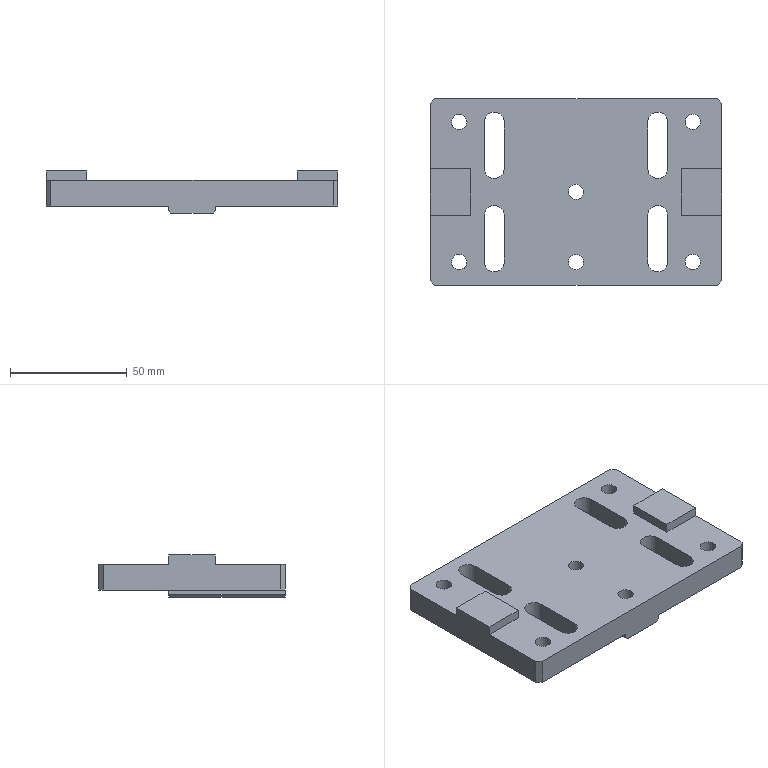NC program | NX | posted with a generic post | part box 125 x 80 x 18 mm
Lines 632 to 1471 of 3483:
(ZLEVEL_PROFILE_1 , TOOL : D6)
N1226 T02 M6
N1228 G54
N1230 G17 G0 G90 X-33.75 Y-10.203 S7000 M3
N1232 G43 Z30. H2
N1234 Z-1.5
N1236 G94 G1 Y-9.818 Z-1.52 F1000.
N1238 X-33.881 Y-9.379 Z-1.544
N1240 X-34.274 Y-8.946 Z-1.575
N1242 X-34.819 Y-8.733 Z-1.606
N1244 X-35.402 Y-8.785 Z-1.636
N1246 X-35.876 Y-9.067 Z-1.665
N1248 X-36.25 Y-9.725 Z-1.705
N1250 Y-30.276 Z-2.782
N1252 X-35.93 Y-30.879 Z-2.818
N1254 X-35.474 Y-31.189 Z-2.846
N1256 X-34.87 Y-31.273 Z-2.878
N1258 X-34.296 Y-31.069 Z-2.91
N1260 X-33.881 Y-30.621 Z-2.942
N1262 X-33.75 Y-30.182 Z-2.966
N1264 Y-20. Z-3.5
N1266 Y-10. F1450.
N1268 G3 X-35. Y-8.75 R1.25
N1270 X-36.25 Y-10. R1.25
N1272 G1 Y-30.
N1274 G3 X-35. Y-31.25 R1.25
N1276 X-33.75 Y-30. R1.25
N1278 G1 Y-20.
N1280 Y-10.452 Z-3.667
N1282 Y-10.153 Z-3.672
N1284 X-33.758 Y-9.855 Z-3.677
N1286 X-33.801 Y-9.645 Z-3.681
N1288 X-33.836 Y-9.545 Z-3.683
N1290 X-33.872 Y-9.462 Z-3.684
N1292 X-33.985 Y-9.315 Z-3.688
N1294 X-34.281 Y-9.006 Z-3.695
N1296 X-34.412 Y-8.923 Z-3.698
N1298 X-34.634 Y-8.832 Z-3.702
N1300 X-34.748 Y-8.796 Z-3.704
N1302 X-34.972 Y-8.771 Z-3.708
N1304 X-35.207 Y-8.791 Z-3.712
N1306 X-35.32 Y-8.815 Z-3.715
N1308 X-35.541 Y-8.894 Z-3.719
N1310 X-35.732 Y-9.014 Z-3.723
N1312 X-35.817 Y-9.086 Z-3.725
N1314 X-35.876 Y-9.144 Z-3.726
N1316 X-35.987 Y-9.268 Z-3.729
N1318 X-36.089 Y-9.432 Z-3.733
N1320 X-36.13 Y-9.519 Z-3.734
N1322 X-36.161 Y-9.612 Z-3.736
N1324 X-36.211 Y-9.803 Z-3.74
N1326 X-36.244 Y-10.098 Z-3.745
N1328 X-36.25 Y-10.396 Z-3.75
N1330 Y-24.718 Z-4.
N1332 Y-30.
N1334 G3 X-35. Y-31.25 R1.25
N1336 X-33.75 Y-30. R1.25
N1338 G1 Y-20.
N1340 Y-10.452 Z-4.167
N1342 Y-10.153 Z-4.172
N1344 X-33.758 Y-9.855 Z-4.177
N1346 X-33.801 Y-9.645 Z-4.181
N1348 X-33.836 Y-9.545 Z-4.183
N1350 X-33.872 Y-9.462 Z-4.184
N1352 X-33.985 Y-9.315 Z-4.188
N1354 X-34.281 Y-9.006 Z-4.195
N1356 X-34.412 Y-8.923 Z-4.198
N1358 X-34.634 Y-8.832 Z-4.202
N1360 X-34.748 Y-8.796 Z-4.204
N1362 X-34.972 Y-8.771 Z-4.208
N1364 X-35.207 Y-8.791 Z-4.212
N1366 X-35.32 Y-8.815 Z-4.215
N1368 X-35.541 Y-8.894 Z-4.219
N1370 X-35.732 Y-9.014 Z-4.223
N1372 X-35.817 Y-9.086 Z-4.225
N1374 X-35.876 Y-9.144 Z-4.226
N1376 X-35.987 Y-9.268 Z-4.229
N1378 X-36.089 Y-9.432 Z-4.233
N1380 X-36.13 Y-9.519 Z-4.234
N1382 X-36.161 Y-9.612 Z-4.236
N1384 X-36.211 Y-9.803 Z-4.24
N1386 X-36.244 Y-10.098 Z-4.245
N1388 X-36.25 Y-10.396 Z-4.25
N1390 Y-24.718 Z-4.5
N1392 Y-30.
N1394 G3 X-35. Y-31.25 R1.25
N1396 X-33.75 Y-30. R1.25
N1398 G1 Y-20.
N1400 Y-10.452 Z-4.667
N1402 Y-10.153 Z-4.672
N1404 X-33.758 Y-9.855 Z-4.677
N1406 X-33.801 Y-9.645 Z-4.681
N1408 X-33.836 Y-9.545 Z-4.683
N1410 X-33.872 Y-9.462 Z-4.684
N1412 X-33.985 Y-9.315 Z-4.688
N1414 X-34.281 Y-9.006 Z-4.695
N1416 X-34.412 Y-8.923 Z-4.698
N1418 X-34.634 Y-8.832 Z-4.702
N1420 X-34.748 Y-8.796 Z-4.704
N1422 X-34.972 Y-8.771 Z-4.708
N1424 X-35.207 Y-8.791 Z-4.712
N1426 X-35.32 Y-8.815 Z-4.715
N1428 X-35.541 Y-8.894 Z-4.719
N1430 X-35.732 Y-9.014 Z-4.723
N1432 X-35.817 Y-9.086 Z-4.725
N1434 X-35.876 Y-9.144 Z-4.726
N1436 X-35.987 Y-9.268 Z-4.729
N1438 X-36.089 Y-9.432 Z-4.733
N1440 X-36.13 Y-9.519 Z-4.734
N1442 X-36.161 Y-9.612 Z-4.736
N1444 X-36.211 Y-9.803 Z-4.74
N1446 X-36.244 Y-10.098 Z-4.745
N1448 X-36.25 Y-10.396 Z-4.75
N1450 Y-24.718 Z-5.
N1452 Y-30.
N1454 G3 X-35. Y-31.25 R1.25
N1456 X-33.75 Y-30. R1.25
N1458 G1 Y-20.
N1460 Y-10.452 Z-5.167
N1462 Y-10.153 Z-5.172
N1464 X-33.758 Y-9.855 Z-5.177
N1466 X-33.801 Y-9.645 Z-5.181
N1468 X-33.836 Y-9.545 Z-5.183
N1470 X-33.872 Y-9.462 Z-5.184
N1472 X-33.985 Y-9.315 Z-5.188
N1474 X-34.281 Y-9.006 Z-5.195
N1476 X-34.412 Y-8.923 Z-5.198
N1478 X-34.634 Y-8.832 Z-5.202
N1480 X-34.748 Y-8.796 Z-5.204
N1482 X-34.972 Y-8.771 Z-5.208
N1484 X-35.207 Y-8.791 Z-5.212
N1486 X-35.32 Y-8.815 Z-5.215
N1488 X-35.541 Y-8.894 Z-5.219
N1490 X-35.732 Y-9.014 Z-5.223
N1492 X-35.817 Y-9.086 Z-5.225
N1494 X-35.876 Y-9.144 Z-5.226
N1496 X-35.987 Y-9.268 Z-5.229
N1498 X-36.089 Y-9.432 Z-5.233
N1500 X-36.13 Y-9.519 Z-5.234
N1502 X-36.161 Y-9.612 Z-5.236
N1504 X-36.211 Y-9.803 Z-5.24
N1506 X-36.243 Y-10.098 Z-5.245
N1508 X-36.25 Y-10.396 Z-5.25
N1510 Y-24.718 Z-5.5
N1512 Y-30.
N1514 G3 X-35. Y-31.25 R1.25
N1516 X-33.75 Y-30. R1.25
N1518 G1 Y-20.
N1520 Y-10.452 Z-5.667
N1522 Y-10.153 Z-5.672
N1524 X-33.758 Y-9.855 Z-5.677
N1526 X-33.801 Y-9.645 Z-5.681
N1528 X-33.836 Y-9.545 Z-5.683
N1530 X-33.872 Y-9.462 Z-5.684
N1532 X-33.985 Y-9.315 Z-5.688
N1534 X-34.281 Y-9.006 Z-5.695
N1536 X-34.412 Y-8.923 Z-5.698
N1538 X-34.634 Y-8.832 Z-5.702
N1540 X-34.748 Y-8.796 Z-5.704
N1542 X-34.972 Y-8.771 Z-5.708
N1544 X-35.207 Y-8.791 Z-5.712
N1546 X-35.32 Y-8.815 Z-5.715
N1548 X-35.541 Y-8.894 Z-5.719
N1550 X-35.732 Y-9.014 Z-5.723
N1552 X-35.817 Y-9.086 Z-5.725
N1554 X-35.876 Y-9.144 Z-5.726
N1556 X-35.987 Y-9.268 Z-5.729
N1558 X-36.089 Y-9.432 Z-5.733
N1560 X-36.13 Y-9.519 Z-5.734
N1562 X-36.161 Y-9.612 Z-5.736
N1564 X-36.211 Y-9.803 Z-5.74
N1566 X-36.243 Y-10.098 Z-5.745
N1568 X-36.25 Y-10.396 Z-5.75
N1570 Y-24.718 Z-6.
N1572 Y-30.
N1574 G3 X-35. Y-31.25 R1.25
N1576 X-33.75 Y-30. R1.25
N1578 G1 Y-20.
N1580 Y-10.452 Z-6.167
N1582 Y-10.153 Z-6.172
N1584 X-33.758 Y-9.855 Z-6.177
N1586 X-33.801 Y-9.645 Z-6.181
N1588 X-33.836 Y-9.545 Z-6.183
N1590 X-33.872 Y-9.462 Z-6.184
N1592 X-33.985 Y-9.315 Z-6.188
N1594 X-34.281 Y-9.006 Z-6.195
N1596 X-34.412 Y-8.923 Z-6.198
N1598 X-34.634 Y-8.832 Z-6.202
N1600 X-34.748 Y-8.796 Z-6.204
N1602 X-34.972 Y-8.771 Z-6.208
N1604 X-35.207 Y-8.791 Z-6.212
N1606 X-35.32 Y-8.815 Z-6.215
N1608 X-35.541 Y-8.894 Z-6.219
N1610 X-35.732 Y-9.014 Z-6.223
N1612 X-35.817 Y-9.086 Z-6.225
N1614 X-35.876 Y-9.144 Z-6.226
N1616 X-35.987 Y-9.268 Z-6.229
N1618 X-36.089 Y-9.432 Z-6.233
N1620 X-36.13 Y-9.519 Z-6.234
N1622 X-36.161 Y-9.612 Z-6.236
N1624 X-36.211 Y-9.803 Z-6.24
N1626 X-36.243 Y-10.098 Z-6.245
N1628 X-36.25 Y-10.396 Z-6.25
N1630 Y-24.718 Z-6.5
N1632 Y-30.
N1634 G3 X-35. Y-31.25 R1.25
N1636 X-33.75 Y-30. R1.25
N1638 G1 Y-20.
N1640 Y-10.452 Z-6.667
N1642 Y-10.153 Z-6.672
N1644 X-33.758 Y-9.855 Z-6.677
N1646 X-33.801 Y-9.645 Z-6.681
N1648 X-33.836 Y-9.545 Z-6.683
N1650 X-33.872 Y-9.462 Z-6.684
N1652 X-33.985 Y-9.315 Z-6.688
N1654 X-34.281 Y-9.006 Z-6.695
N1656 X-34.412 Y-8.923 Z-6.698
N1658 X-34.634 Y-8.832 Z-6.702
N1660 X-34.748 Y-8.796 Z-6.704
N1662 X-34.972 Y-8.771 Z-6.708
N1664 X-35.207 Y-8.791 Z-6.712
N1666 X-35.32 Y-8.815 Z-6.715
N1668 X-35.541 Y-8.894 Z-6.719
N1670 X-35.732 Y-9.014 Z-6.723
N1672 X-35.817 Y-9.086 Z-6.725
N1674 X-35.876 Y-9.144 Z-6.726
N1676 X-35.987 Y-9.268 Z-6.729
N1678 X-36.089 Y-9.432 Z-6.733
N1680 X-36.13 Y-9.519 Z-6.734
N1682 X-36.161 Y-9.612 Z-6.736
N1684 X-36.211 Y-9.803 Z-6.74
N1686 X-36.243 Y-10.098 Z-6.745
N1688 X-36.25 Y-10.396 Z-6.75
N1690 Y-24.718 Z-7.
N1692 Y-30.
N1694 G3 X-35. Y-31.25 R1.25
N1696 X-33.75 Y-30. R1.25
N1698 G1 Y-20.
N1700 Y-10.452 Z-7.167
N1702 Y-10.153 Z-7.172
N1704 X-33.758 Y-9.855 Z-7.177
N1706 X-33.801 Y-9.645 Z-7.181
N1708 X-33.836 Y-9.545 Z-7.183
N1710 X-33.872 Y-9.462 Z-7.184
N1712 X-33.985 Y-9.315 Z-7.188
N1714 X-34.281 Y-9.006 Z-7.195
N1716 X-34.412 Y-8.923 Z-7.198
N1718 X-34.634 Y-8.832 Z-7.202
N1720 X-34.748 Y-8.796 Z-7.204
N1722 X-34.972 Y-8.771 Z-7.208
N1724 X-35.207 Y-8.791 Z-7.212
N1726 X-35.32 Y-8.815 Z-7.215
N1728 X-35.541 Y-8.894 Z-7.219
N1730 X-35.732 Y-9.014 Z-7.223
N1732 X-35.817 Y-9.086 Z-7.225
N1734 X-35.876 Y-9.144 Z-7.226
N1736 X-35.987 Y-9.268 Z-7.229
N1738 X-36.089 Y-9.432 Z-7.233
N1740 X-36.13 Y-9.519 Z-7.234
N1742 X-36.161 Y-9.612 Z-7.236
N1744 X-36.211 Y-9.803 Z-7.24
N1746 X-36.243 Y-10.098 Z-7.245
N1748 X-36.25 Y-10.396 Z-7.25
N1750 Y-24.718 Z-7.5
N1752 Y-30.
N1754 G3 X-35. Y-31.25 R1.25
N1756 X-33.75 Y-30. R1.25
N1758 G1 Y-20.
N1760 Y-10.452 Z-7.667
N1762 Y-10.153 Z-7.672
N1764 X-33.758 Y-9.855 Z-7.677
N1766 X-33.801 Y-9.645 Z-7.681
N1768 X-33.836 Y-9.545 Z-7.683
N1770 X-33.872 Y-9.462 Z-7.684
N1772 X-33.985 Y-9.315 Z-7.688
N1774 X-34.281 Y-9.006 Z-7.695
N1776 X-34.412 Y-8.923 Z-7.698
N1778 X-34.634 Y-8.832 Z-7.702
N1780 X-34.748 Y-8.796 Z-7.704
N1782 X-34.972 Y-8.771 Z-7.708
N1784 X-35.207 Y-8.791 Z-7.712
N1786 X-35.32 Y-8.815 Z-7.715
N1788 X-35.541 Y-8.894 Z-7.719
N1790 X-35.732 Y-9.014 Z-7.723
N1792 X-35.817 Y-9.086 Z-7.725
N1794 X-35.876 Y-9.144 Z-7.726
N1796 X-35.987 Y-9.268 Z-7.729
N1798 X-36.089 Y-9.432 Z-7.733
N1800 X-36.13 Y-9.519 Z-7.734
N1802 X-36.161 Y-9.612 Z-7.736
N1804 X-36.211 Y-9.803 Z-7.74
N1806 X-36.243 Y-10.098 Z-7.745
N1808 X-36.25 Y-10.396 Z-7.75
N1810 Y-24.718 Z-8.
N1812 Y-30.
N1814 G3 X-35. Y-31.25 R1.25
N1816 X-33.75 Y-30. R1.25
N1818 G1 Y-20.
N1820 Y-10.452 Z-8.167
N1822 Y-10.153 Z-8.172
N1824 X-33.758 Y-9.855 Z-8.177
N1826 X-33.801 Y-9.645 Z-8.181
N1828 X-33.836 Y-9.545 Z-8.183
N1830 X-33.872 Y-9.462 Z-8.184
N1832 X-33.985 Y-9.315 Z-8.188
N1834 X-34.281 Y-9.006 Z-8.195
N1836 X-34.412 Y-8.923 Z-8.198
N1838 X-34.634 Y-8.832 Z-8.202
N1840 X-34.748 Y-8.796 Z-8.204
N1842 X-34.972 Y-8.771 Z-8.208
N1844 X-35.207 Y-8.791 Z-8.212
N1846 X-35.32 Y-8.815 Z-8.215
N1848 X-35.541 Y-8.894 Z-8.219
N1850 X-35.732 Y-9.014 Z-8.223
N1852 X-35.817 Y-9.086 Z-8.225
N1854 X-35.876 Y-9.144 Z-8.226
N1856 X-35.987 Y-9.268 Z-8.229
N1858 X-36.089 Y-9.432 Z-8.233
N1860 X-36.13 Y-9.519 Z-8.234
N1862 X-36.161 Y-9.612 Z-8.236
N1864 X-36.211 Y-9.803 Z-8.24
N1866 X-36.243 Y-10.098 Z-8.245
N1868 X-36.25 Y-10.396 Z-8.25
N1870 Y-24.718 Z-8.5
N1872 Y-30.
N1874 G3 X-35. Y-31.25 R1.25
N1876 X-33.75 Y-30. R1.25
N1878 G1 Y-20.
N1880 Y-10.452 Z-8.667
N1882 Y-10.153 Z-8.672
N1884 X-33.758 Y-9.855 Z-8.677
N1886 X-33.801 Y-9.645 Z-8.681
N1888 X-33.836 Y-9.545 Z-8.683
N1890 X-33.872 Y-9.462 Z-8.684
N1892 X-33.985 Y-9.315 Z-8.688
N1894 X-34.281 Y-9.006 Z-8.695
N1896 X-34.412 Y-8.923 Z-8.698
N1898 X-34.634 Y-8.832 Z-8.702
N1900 X-34.748 Y-8.796 Z-8.704
N1902 X-34.972 Y-8.771 Z-8.708
N1904 X-35.207 Y-8.791 Z-8.712
N1906 X-35.32 Y-8.815 Z-8.715
N1908 X-35.541 Y-8.894 Z-8.719
N1910 X-35.732 Y-9.014 Z-8.723
N1912 X-35.817 Y-9.086 Z-8.725
N1914 X-35.876 Y-9.144 Z-8.726
N1916 X-35.987 Y-9.268 Z-8.729
N1918 X-36.089 Y-9.432 Z-8.733
N1920 X-36.13 Y-9.519 Z-8.734
N1922 X-36.161 Y-9.612 Z-8.736
N1924 X-36.211 Y-9.803 Z-8.74
N1926 X-36.243 Y-10.098 Z-8.745
N1928 X-36.25 Y-10.396 Z-8.75
N1930 Y-24.718 Z-9.
N1932 Y-30.
N1934 G3 X-35. Y-31.25 R1.25
N1936 X-33.75 Y-30. R1.25
N1938 G1 Y-20.
N1940 Y-10.452 Z-9.167
N1942 Y-10.153 Z-9.172
N1944 X-33.758 Y-9.855 Z-9.177
N1946 X-33.801 Y-9.645 Z-9.181
N1948 X-33.836 Y-9.545 Z-9.183
N1950 X-33.871 Y-9.462 Z-9.184
N1952 X-33.985 Y-9.315 Z-9.188
N1954 X-34.281 Y-9.006 Z-9.195
N1956 X-34.412 Y-8.923 Z-9.198
N1958 X-34.634 Y-8.832 Z-9.202
N1960 X-34.748 Y-8.796 Z-9.204
N1962 X-34.972 Y-8.771 Z-9.208
N1964 X-35.207 Y-8.791 Z-9.212
N1966 X-35.32 Y-8.815 Z-9.215
N1968 X-35.541 Y-8.894 Z-9.219
N1970 X-35.732 Y-9.014 Z-9.223
N1972 X-35.817 Y-9.086 Z-9.225
N1974 X-35.876 Y-9.144 Z-9.226
N1976 X-35.987 Y-9.268 Z-9.229
N1978 X-36.089 Y-9.432 Z-9.233
N1980 X-36.13 Y-9.519 Z-9.234
N1982 X-36.161 Y-9.612 Z-9.236
N1984 X-36.211 Y-9.803 Z-9.24
N1986 X-36.243 Y-10.098 Z-9.245
N1988 X-36.25 Y-10.396 Z-9.25
N1990 Y-24.718 Z-9.5
N1992 Y-30.
N1994 G3 X-35. Y-31.25 R1.25
N1996 X-33.75 Y-30. R1.25
N1998 G1 Y-20.
N2000 Y-10.452 Z-9.667
N2002 Y-10.153 Z-9.672
N2004 X-33.758 Y-9.855 Z-9.677
N2006 X-33.801 Y-9.645 Z-9.681
N2008 X-33.836 Y-9.545 Z-9.683
N2010 X-33.871 Y-9.462 Z-9.684
N2012 X-33.985 Y-9.315 Z-9.688
N2014 X-34.281 Y-9.006 Z-9.695
N2016 X-34.412 Y-8.923 Z-9.698
N2018 X-34.634 Y-8.832 Z-9.702
N2020 X-34.748 Y-8.796 Z-9.704
N2022 X-34.972 Y-8.771 Z-9.708
N2024 X-35.207 Y-8.791 Z-9.712
N2026 X-35.32 Y-8.815 Z-9.715
N2028 X-35.541 Y-8.894 Z-9.719
N2030 X-35.732 Y-9.014 Z-9.723
N2032 X-35.817 Y-9.086 Z-9.725
N2034 X-35.876 Y-9.144 Z-9.726
N2036 X-35.987 Y-9.268 Z-9.729
N2038 X-36.089 Y-9.432 Z-9.733
N2040 X-36.13 Y-9.519 Z-9.734
N2042 X-36.161 Y-9.612 Z-9.736
N2044 X-36.211 Y-9.803 Z-9.74
N2046 X-36.243 Y-10.098 Z-9.745
N2048 X-36.25 Y-10.396 Z-9.75
N2050 Y-24.718 Z-10.
N2052 Y-30.
N2054 G3 X-35. Y-31.25 R1.25
N2056 X-33.75 Y-30. R1.25
N2058 G1 Y-20.
N2060 Y-10.452 Z-10.167
N2062 Y-10.153 Z-10.172
N2064 X-33.758 Y-9.855 Z-10.177
N2066 X-33.801 Y-9.645 Z-10.181
N2068 X-33.836 Y-9.545 Z-10.183
N2070 X-33.871 Y-9.462 Z-10.184
N2072 X-33.985 Y-9.315 Z-10.188
N2074 X-34.281 Y-9.006 Z-10.195
N2076 X-34.412 Y-8.924 Z-10.198
N2078 X-34.634 Y-8.832 Z-10.202
N2080 X-34.748 Y-8.796 Z-10.204
N2082 X-34.972 Y-8.771 Z-10.208
N2084 X-35.207 Y-8.791 Z-10.212
N2086 X-35.32 Y-8.815 Z-10.215
N2088 X-35.541 Y-8.894 Z-10.219
N2090 X-35.732 Y-9.014 Z-10.223
N2092 X-35.817 Y-9.086 Z-10.225
N2094 X-35.876 Y-9.144 Z-10.226
N2096 X-35.987 Y-9.268 Z-10.229
N2098 X-36.089 Y-9.432 Z-10.233
N2100 X-36.13 Y-9.519 Z-10.234
N2102 X-36.161 Y-9.612 Z-10.236
N2104 X-36.211 Y-9.803 Z-10.24
N2106 X-36.243 Y-10.098 Z-10.245
N2108 X-36.25 Y-10.396 Z-10.25
N2110 Y-24.718 Z-10.5
N2112 Y-30.
N2114 G3 X-35. Y-31.25 R1.25
N2116 X-33.75 Y-30. R1.25
N2118 G1 Y-20.
N2120 Y-10.452 Z-10.667
N2122 Y-10.153 Z-10.672
N2124 X-33.758 Y-9.855 Z-10.677
N2126 X-33.801 Y-9.645 Z-10.681
N2128 X-33.836 Y-9.545 Z-10.683
N2130 X-33.871 Y-9.462 Z-10.684
N2132 X-33.985 Y-9.315 Z-10.688
N2134 X-34.281 Y-9.006 Z-10.695
N2136 X-34.412 Y-8.924 Z-10.698
N2138 X-34.634 Y-8.832 Z-10.702
N2140 X-34.748 Y-8.796 Z-10.704
N2142 X-34.972 Y-8.771 Z-10.708
N2144 X-35.207 Y-8.791 Z-10.712
N2146 X-35.32 Y-8.815 Z-10.715
N2148 X-35.541 Y-8.894 Z-10.719
N2150 X-35.732 Y-9.014 Z-10.723
N2152 X-35.817 Y-9.086 Z-10.725
N2154 X-35.876 Y-9.144 Z-10.726
N2156 X-35.987 Y-9.268 Z-10.729
N2158 X-36.089 Y-9.432 Z-10.733
N2160 X-36.13 Y-9.519 Z-10.734
N2162 X-36.161 Y-9.612 Z-10.736
N2164 X-36.211 Y-9.803 Z-10.74
N2166 X-36.243 Y-10.098 Z-10.745
N2168 X-36.25 Y-10.396 Z-10.75
N2170 Y-24.718 Z-11.
N2172 Y-30.
N2174 G3 X-35. Y-31.25 R1.25
N2176 X-33.75 Y-30. R1.25
N2178 G1 Y-20.
N2180 Y-10.452 Z-11.167
N2182 Y-10.153 Z-11.172
N2184 X-33.758 Y-9.855 Z-11.177
N2186 X-33.801 Y-9.645 Z-11.181
N2188 X-33.836 Y-9.545 Z-11.183
N2190 X-33.871 Y-9.462 Z-11.184
N2192 X-33.985 Y-9.315 Z-11.188
N2194 X-34.281 Y-9.006 Z-11.195
N2196 X-34.412 Y-8.924 Z-11.198
N2198 X-34.634 Y-8.832 Z-11.202
N2200 X-34.748 Y-8.796 Z-11.204
N2202 X-34.972 Y-8.771 Z-11.208
N2204 X-35.207 Y-8.791 Z-11.212
N2206 X-35.32 Y-8.815 Z-11.215
N2208 X-35.541 Y-8.894 Z-11.219
N2210 X-35.732 Y-9.014 Z-11.223
N2212 X-35.817 Y-9.086 Z-11.225
N2214 X-35.875 Y-9.144 Z-11.226
N2216 X-35.987 Y-9.268 Z-11.229
N2218 X-36.088 Y-9.432 Z-11.233
N2220 X-36.13 Y-9.519 Z-11.234
N2222 X-36.161 Y-9.612 Z-11.236
N2224 X-36.211 Y-9.803 Z-11.24
N2226 X-36.243 Y-10.098 Z-11.245
N2228 X-36.25 Y-10.396 Z-11.25
N2230 Y-24.718 Z-11.5
N2232 Y-30.
N2234 G3 X-35. Y-31.25 R1.25
N2236 X-33.75 Y-30. R1.25
N2238 G1 Y-20.
N2240 Y-10.452 Z-11.667
N2242 Y-10.153 Z-11.672
N2244 X-33.758 Y-9.855 Z-11.677
N2246 X-33.801 Y-9.645 Z-11.681
N2248 X-33.836 Y-9.545 Z-11.683
N2250 X-33.871 Y-9.462 Z-11.684
N2252 X-33.985 Y-9.315 Z-11.688
N2254 X-34.281 Y-9.006 Z-11.695
N2256 X-34.412 Y-8.924 Z-11.698
N2258 X-34.634 Y-8.832 Z-11.702
N2260 X-34.748 Y-8.796 Z-11.704
N2262 X-34.972 Y-8.771 Z-11.708
N2264 X-35.207 Y-8.791 Z-11.712
N2266 X-35.32 Y-8.815 Z-11.715
N2268 X-35.541 Y-8.894 Z-11.719
N2270 X-35.732 Y-9.014 Z-11.723
N2272 X-35.817 Y-9.086 Z-11.725
N2274 X-35.875 Y-9.144 Z-11.726
N2276 X-35.987 Y-9.268 Z-11.729
N2278 X-36.088 Y-9.432 Z-11.733
N2280 X-36.13 Y-9.519 Z-11.734
N2282 X-36.161 Y-9.612 Z-11.736
N2284 X-36.211 Y-9.803 Z-11.74
N2286 X-36.243 Y-10.098 Z-11.745
N2288 X-36.25 Y-10.396 Z-11.75
N2290 Y-24.718 Z-12.
N2292 Y-30.
N2294 G3 X-35. Y-31.25 R1.25
N2296 X-33.75 Y-30. R1.25
N2298 G1 Y-20.
N2300 Y-10.452 Z-12.167
N2302 Y-10.153 Z-12.172
N2304 X-33.758 Y-9.855 Z-12.177
N2306 X-33.801 Y-9.645 Z-12.181
N2308 X-33.836 Y-9.545 Z-12.183
N2310 X-33.871 Y-9.462 Z-12.184
N2312 X-33.985 Y-9.315 Z-12.188
N2314 X-34.281 Y-9.006 Z-12.195
N2316 X-34.412 Y-8.924 Z-12.198
N2318 X-34.634 Y-8.832 Z-12.202
N2320 X-34.748 Y-8.796 Z-12.204
N2322 X-34.972 Y-8.771 Z-12.208
N2324 X-35.207 Y-8.791 Z-12.212
N2326 X-35.32 Y-8.815 Z-12.215
N2328 X-35.541 Y-8.894 Z-12.219
N2330 X-35.732 Y-9.014 Z-12.223
N2332 X-35.817 Y-9.086 Z-12.225
N2334 X-35.875 Y-9.144 Z-12.226
N2336 X-35.987 Y-9.268 Z-12.229
N2338 X-36.088 Y-9.432 Z-12.233
N2340 X-36.13 Y-9.519 Z-12.234
N2342 X-36.161 Y-9.612 Z-12.236
N2344 X-36.211 Y-9.803 Z-12.24
N2346 X-36.243 Y-10.098 Z-12.245
N2348 X-36.25 Y-10.396 Z-12.25
N2350 Y-24.718 Z-12.5
N2352 Y-30.
N2354 G3 X-35. Y-31.25 R1.25
N2356 X-33.75 Y-30. R1.25
N2358 G1 Y-20.
N2360 Y-10.452 Z-12.667
N2362 Y-10.153 Z-12.672
N2364 X-33.758 Y-9.855 Z-12.677
N2366 X-33.801 Y-9.645 Z-12.681
N2368 X-33.836 Y-9.545 Z-12.683
N2370 X-33.871 Y-9.462 Z-12.684
N2372 X-33.985 Y-9.315 Z-12.688
N2374 X-34.281 Y-9.006 Z-12.695
N2376 X-34.412 Y-8.924 Z-12.698
N2378 X-34.634 Y-8.832 Z-12.702
N2380 X-34.748 Y-8.796 Z-12.704
N2382 X-34.972 Y-8.771 Z-12.708
N2384 X-35.207 Y-8.791 Z-12.712
N2386 X-35.32 Y-8.815 Z-12.715
N2388 X-35.541 Y-8.894 Z-12.719
N2390 X-35.732 Y-9.014 Z-12.723
N2392 X-35.817 Y-9.086 Z-12.725
N2394 X-35.875 Y-9.144 Z-12.726
N2396 X-35.987 Y-9.268 Z-12.729
N2398 X-36.088 Y-9.432 Z-12.733
N2400 X-36.13 Y-9.519 Z-12.734
N2402 X-36.161 Y-9.612 Z-12.736
N2404 X-36.211 Y-9.803 Z-12.74
N2406 X-36.243 Y-10.098 Z-12.745
N2408 X-36.25 Y-10.396 Z-12.75
N2410 Y-24.718 Z-13.
N2412 Y-30.
N2414 G3 X-35. Y-31.25 R1.25
N2416 X-33.75 Y-30. R1.25
N2418 G1 Y-20.
N2420 Y-10.452 Z-13.167
N2422 Y-10.153 Z-13.172
N2424 X-33.758 Y-9.855 Z-13.177
N2426 X-33.801 Y-9.645 Z-13.181
N2428 X-33.836 Y-9.545 Z-13.183
N2430 X-33.871 Y-9.462 Z-13.184
N2432 X-33.985 Y-9.315 Z-13.188
N2434 X-34.282 Y-9.006 Z-13.195
N2436 X-34.412 Y-8.924 Z-13.198
N2438 X-34.634 Y-8.832 Z-13.202
N2440 X-34.748 Y-8.796 Z-13.204
N2442 X-34.972 Y-8.771 Z-13.208
N2444 X-35.207 Y-8.791 Z-13.212
N2446 X-35.32 Y-8.815 Z-13.215
N2448 X-35.541 Y-8.894 Z-13.219
N2450 X-35.732 Y-9.014 Z-13.223
N2452 X-35.817 Y-9.086 Z-13.225
N2454 X-35.875 Y-9.144 Z-13.226
N2456 X-35.987 Y-9.268 Z-13.229
N2458 X-36.088 Y-9.432 Z-13.233
N2460 X-36.13 Y-9.519 Z-13.234
N2462 X-36.161 Y-9.612 Z-13.236
N2464 X-36.211 Y-9.803 Z-13.24
N2466 X-36.243 Y-10.098 Z-13.245
N2468 X-36.25 Y-10.396 Z-13.25
N2470 Y-24.718 Z-13.5
N2472 Y-30.
N2474 G3 X-35. Y-31.25 R1.25
N2476 X-33.75 Y-30. R1.25
N2478 G1 Y-20.
N2480 Y-10.452 Z-13.667
N2482 Y-10.153 Z-13.672
N2484 X-33.758 Y-9.855 Z-13.677
N2486 X-33.801 Y-9.645 Z-13.681
N2488 X-33.836 Y-9.545 Z-13.683
N2490 X-33.871 Y-9.462 Z-13.684
N2492 X-33.985 Y-9.315 Z-13.688
N2494 X-34.282 Y-9.006 Z-13.695
N2496 X-34.412 Y-8.924 Z-13.698
N2498 X-34.634 Y-8.832 Z-13.702
N2500 X-34.748 Y-8.796 Z-13.704
N2502 X-34.972 Y-8.771 Z-13.708
N2504 X-35.207 Y-8.791 Z-13.712
N2506 X-35.32 Y-8.815 Z-13.715
N2508 X-35.541 Y-8.894 Z-13.719
N2510 X-35.732 Y-9.014 Z-13.723
N2512 X-35.817 Y-9.086 Z-13.725
N2514 X-35.987 Y-9.268 Z-13.729
N2516 X-36.088 Y-9.432 Z-13.733
N2518 X-36.13 Y-9.519 Z-13.734
N2520 X-36.161 Y-9.612 Z-13.736
N2522 X-36.211 Y-9.803 Z-13.74
N2524 X-36.243 Y-10.098 Z-13.745
N2526 X-36.25 Y-10.396 Z-13.75
N2528 Y-24.718 Z-14.
N2530 Y-30.
N2532 G3 X-35. Y-31.25 R1.25
N2534 X-33.75 Y-30. R1.25
N2536 G1 Y-10.
N2538 G3 X-35. Y-8.75 R1.25
N2540 X-36.25 Y-10. R1.25
N2542 G1 Y-24.718
N2544 Z-12.5
N2546 G0 Z30.
N2548 X-33.75 Y29.797
N2550 Z-1.5
N2552 G1 Y30.182 Z-1.52 F1000.
N2554 X-33.881 Y30.621 Z-1.544
N2556 X-34.296 Y31.069 Z-1.576
N2558 X-34.87 Y31.273 Z-1.608
N2560 X-35.474 Y31.189 Z-1.64
N2562 X-35.93 Y30.879 Z-1.669
N2564 X-36.25 Y30.276 Z-1.705
N2566 Y9.725 Z-2.782
N2568 X-35.876 Y9.067 Z-2.821
N2570 X-35.402 Y8.785 Z-2.85
N2572 X-34.819 Y8.733 Z-2.881
N2574 X-34.274 Y8.946 Z-2.912
N2576 X-33.881 Y9.379 Z-2.942
N2578 X-33.75 Y9.818 Z-2.966
N2580 Y20. Z-3.5
N2582 Y30. F1450.
N2584 G3 X-35. Y31.25 R1.25
N2586 X-36.25 Y30. R1.25
N2588 G1 Y10.
N2590 G3 X-35. Y8.75 R1.25
N2592 X-33.75 Y10. R1.25
N2594 G1 Y20.
N2596 Y29.548 Z-3.667
N2598 X-33.774 Y30.046 Z-3.675
N2600 X-33.784 Y30.142 Z-3.677
N2602 X-33.839 Y30.392 Z-3.682
N2604 X-33.881 Y30.511 Z-3.684
N2606 X-33.985 Y30.685 Z-3.688
N2608 X-34.146 Y30.877 Z-3.692
N2610 X-34.234 Y30.964 Z-3.694
N2612 X-34.412 Y31.077 Z-3.698
N2614 X-34.635 Y31.169 Z-3.702
N2616 X-34.749 Y31.204 Z-3.704
N2618 X-34.972 Y31.229 Z-3.708
N2620 X-35.207 Y31.209 Z-3.712
N2622 X-35.32 Y31.185 Z-3.715
N2624 X-35.541 Y31.106 Z-3.719
N2626 X-35.732 Y30.986 Z-3.723
N2628 X-35.817 Y30.914 Z-3.725
N2630 X-35.876 Y30.856 Z-3.726
N2632 X-35.987 Y30.732 Z-3.729
N2634 X-36.089 Y30.568 Z-3.733
N2636 X-36.13 Y30.481 Z-3.734
N2638 X-36.161 Y30.388 Z-3.736
N2640 X-36.211 Y30.197 Z-3.74
N2642 X-36.244 Y29.902 Z-3.745
N2644 X-36.25 Y29.605 Z-3.75
N2646 Y15.282 Z-4.
N2648 Y10.
N2650 G3 X-35. Y8.75 R1.25
N2652 X-33.75 Y10. R1.25
N2654 G1 Y20.
N2656 Y29.548 Z-4.167
N2658 X-33.774 Y30.046 Z-4.175
N2660 X-33.784 Y30.142 Z-4.177
N2662 X-33.839 Y30.392 Z-4.182
N2664 X-33.881 Y30.511 Z-4.184
N2666 X-33.985 Y30.685 Z-4.188
N2668 X-34.146 Y30.877 Z-4.192
N2670 X-34.234 Y30.964 Z-4.194
N2672 X-34.412 Y31.077 Z-4.198
N2674 X-34.635 Y31.169 Z-4.202
N2676 X-34.749 Y31.204 Z-4.204
N2678 X-34.972 Y31.229 Z-4.208
N2680 X-35.207 Y31.209 Z-4.212
N2682 X-35.32 Y31.185 Z-4.215
N2684 X-35.541 Y31.106 Z-4.219
N2686 X-35.732 Y30.986 Z-4.223
N2688 X-35.817 Y30.914 Z-4.225
N2690 X-35.876 Y30.856 Z-4.226
N2692 X-35.987 Y30.732 Z-4.229
N2694 X-36.089 Y30.568 Z-4.233
N2696 X-36.13 Y30.481 Z-4.234
N2698 X-36.161 Y30.388 Z-4.236
N2700 X-36.211 Y30.197 Z-4.24
N2702 X-36.244 Y29.902 Z-4.245
N2704 X-36.25 Y29.605 Z-4.25
N2706 Y15.282 Z-4.5
N2708 Y10.
N2710 G3 X-35. Y8.75 R1.25
N2712 X-33.75 Y10. R1.25
N2714 G1 Y20.
N2716 Y29.548 Z-4.667
N2718 X-33.774 Y30.046 Z-4.675
N2720 X-33.784 Y30.142 Z-4.677
N2722 X-33.839 Y30.392 Z-4.682
N2724 X-33.881 Y30.511 Z-4.684
N2726 X-33.985 Y30.685 Z-4.688
N2728 X-34.146 Y30.877 Z-4.692
N2730 X-34.234 Y30.964 Z-4.694
N2732 X-34.412 Y31.077 Z-4.698
N2734 X-34.635 Y31.169 Z-4.702
N2736 X-34.749 Y31.204 Z-4.704
N2738 X-34.972 Y31.229 Z-4.708
N2740 X-35.207 Y31.209 Z-4.712
N2742 X-35.32 Y31.185 Z-4.715
N2744 X-35.541 Y31.106 Z-4.719
N2746 X-35.732 Y30.986 Z-4.723
N2748 X-35.817 Y30.914 Z-4.725
N2750 X-35.876 Y30.856 Z-4.726
N2752 X-35.987 Y30.732 Z-4.729
N2754 X-36.089 Y30.568 Z-4.733
N2756 X-36.13 Y30.481 Z-4.734
N2758 X-36.161 Y30.388 Z-4.736
N2760 X-36.211 Y30.197 Z-4.74
N2762 X-36.244 Y29.902 Z-4.745
N2764 X-36.25 Y29.605 Z-4.75
N2766 Y15.282 Z-5.
N2768 Y10.
N2770 G3 X-35. Y8.75 R1.25
N2772 X-33.75 Y10. R1.25
N2774 G1 Y20.
N2776 Y29.548 Z-5.167
N2778 X-33.774 Y30.046 Z-5.175
N2780 X-33.784 Y30.142 Z-5.177
N2782 X-33.839 Y30.392 Z-5.182
N2784 X-33.881 Y30.511 Z-5.184
N2786 X-33.985 Y30.685 Z-5.188
N2788 X-34.146 Y30.877 Z-5.192
N2790 X-34.234 Y30.964 Z-5.194
N2792 X-34.412 Y31.077 Z-5.198
N2794 X-34.635 Y31.169 Z-5.202
N2796 X-34.749 Y31.204 Z-5.204
N2798 X-34.972 Y31.229 Z-5.208
N2800 X-35.207 Y31.209 Z-5.212
N2802 X-35.32 Y31.185 Z-5.215
N2804 X-35.541 Y31.106 Z-5.219
N2806 X-35.732 Y30.986 Z-5.223
N2808 X-35.817 Y30.914 Z-5.225
N2810 X-35.876 Y30.856 Z-5.226
N2812 X-35.987 Y30.732 Z-5.229
N2814 X-36.089 Y30.568 Z-5.233
N2816 X-36.13 Y30.481 Z-5.234
N2818 X-36.161 Y30.388 Z-5.236
N2820 X-36.211 Y30.197 Z-5.24
N2822 X-36.243 Y29.902 Z-5.245
N2824 X-36.25 Y29.605 Z-5.25
N2826 Y15.282 Z-5.5
N2828 Y10.
N2830 G3 X-35. Y8.75 R1.25
N2832 X-33.75 Y10. R1.25
N2834 G1 Y20.
N2836 Y29.548 Z-5.667
N2838 X-33.774 Y30.046 Z-5.675
N2840 X-33.784 Y30.142 Z-5.677
N2842 X-33.839 Y30.392 Z-5.682
N2844 X-33.881 Y30.511 Z-5.684
N2846 X-33.985 Y30.685 Z-5.688
N2848 X-34.146 Y30.877 Z-5.692
N2850 X-34.234 Y30.964 Z-5.694
N2852 X-34.412 Y31.077 Z-5.698
N2854 X-34.635 Y31.169 Z-5.702
N2856 X-34.749 Y31.204 Z-5.704
N2858 X-34.972 Y31.229 Z-5.708
N2860 X-35.207 Y31.209 Z-5.712
N2862 X-35.32 Y31.185 Z-5.715
N2864 X-35.541 Y31.106 Z-5.719
N2866 X-35.732 Y30.986 Z-5.723
N2868 X-35.817 Y30.914 Z-5.725
N2870 X-35.876 Y30.856 Z-5.726
N2872 X-35.987 Y30.732 Z-5.729
N2874 X-36.089 Y30.568 Z-5.733
N2876 X-36.13 Y30.481 Z-5.734
N2878 X-36.161 Y30.388 Z-5.736
N2880 X-36.211 Y30.197 Z-5.74
N2882 X-36.243 Y29.902 Z-5.745
N2884 X-36.25 Y29.605 Z-5.75
N2886 Y15.282 Z-6.
N2888 Y10.
N2890 G3 X-35. Y8.75 R1.25
N2892 X-33.75 Y10. R1.25
N2894 G1 Y20.
N2896 Y29.548 Z-6.167
N2898 X-33.774 Y30.046 Z-6.175